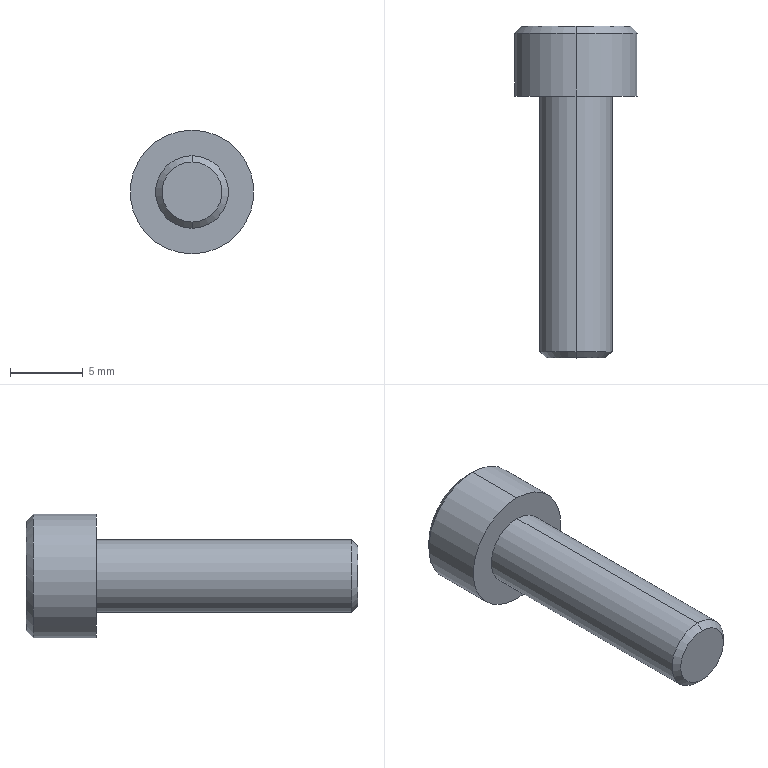Part | STEP file | 0244_Z_008_MFJC44-20-20_3 | 1 solid | 25 faces | box 8.5 x 22.82 x 8.5 mm | volume 582.868 mm3 | plane 15 | cone 6 | cylinder 4 | commonest cylinder face diameters 5 x2 8.5 x2